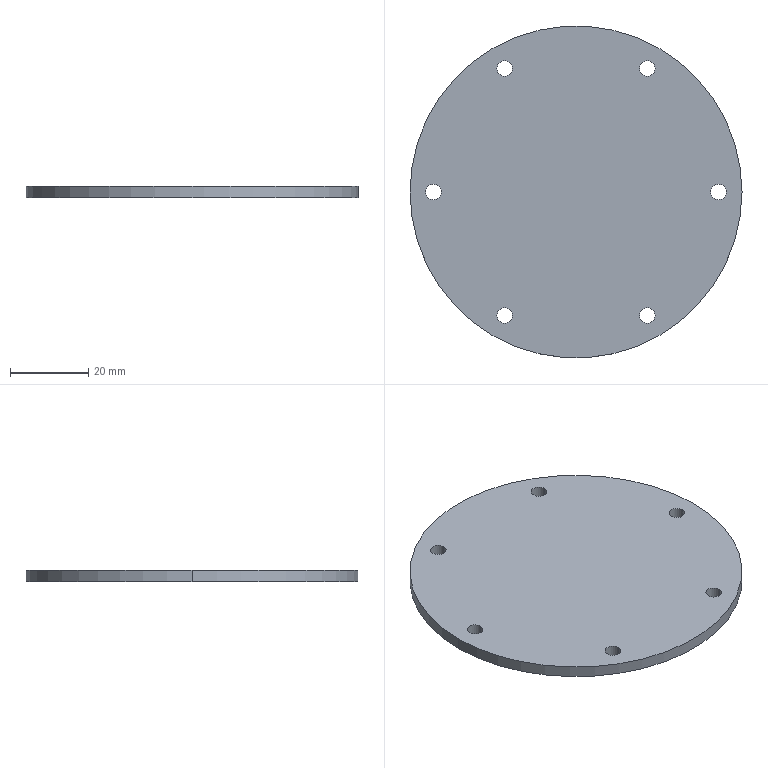Part | SolidWorks | features FlatPattern 1, SMBaseFlange 1, SheetMetal 1 | 1 solid | 16 faces | box 85 x 85 x 3 mm | volume 16797 mm3 | cylinder 14 | plane 2 | commonest cylinder face diameters 4 x12 85 x2
STEP:
#1=CARTESIAN_POINT('',(500.89,-193.14,3.));
#2=VERTEX_POINT('',#1);
#3=CARTESIAN_POINT('',(504.89,-193.14,3.));
#4=VERTEX_POINT('',#3);
#5=CARTESIAN_POINT('',(502.89,-193.14,3.));
#6=DIRECTION('',(0.,0.,1.));
#7=DIRECTION('',(1.,0.,0.));
#8=AXIS2_PLACEMENT_3D('',#5,#6,#7);
#9=CIRCLE('',#8,2.);
#10=EDGE_CURVE('',#2,#4,#9,.T.);
#11=ORIENTED_EDGE('',*,*,#10,.T.);
#12=CARTESIAN_POINT('',(504.89,-193.14,0.));
#13=VERTEX_POINT('',#12);
#14=CARTESIAN_POINT('',(504.89,-193.14,3.));
#15=DIRECTION('',(0.,0.,-1.));
#16=VECTOR('',#15,1000.);
#17=LINE('',#14,#16);
#18=EDGE_CURVE('',#4,#13,#17,.T.);
#19=ORIENTED_EDGE('',*,*,#18,.T.);
#20=CARTESIAN_POINT('',(500.89,-193.14,0.));
#21=VERTEX_POINT('',#20);
#22=CARTESIAN_POINT('',(502.89,-193.14,0.));
#23=DIRECTION('',(0.,0.,1.));
#24=DIRECTION('',(1.,0.,0.));
#25=AXIS2_PLACEMENT_3D('',#22,#23,#24);
#26=CIRCLE('',#25,2.);
#27=EDGE_CURVE('',#21,#13,#26,.T.);
#28=ORIENTED_EDGE('',*,*,#27,.F.);
#29=CARTESIAN_POINT('',(500.89,-193.14,3.));
#30=DIRECTION('',(0.,0.,-1.));
#31=VECTOR('',#30,1000.);
#32=LINE('',#29,#31);
#33=EDGE_CURVE('',#2,#21,#32,.T.);
#34=ORIENTED_EDGE('',*,*,#33,.F.);
#35=EDGE_LOOP('',(#11,#19,#28,#34));
#36=FACE_OUTER_BOUND('',#35,.T.);
#37=CARTESIAN_POINT('',(502.89,-193.14,3.));
#38=DIRECTION('',(0.,0.,-1.));
#39=DIRECTION('',(-1.,0.,0.));
#40=AXIS2_PLACEMENT_3D('',#37,#38,#39);
#41=CYLINDRICAL_SURFACE('',#40,2.);
#42=ADVANCED_FACE('',(#36),#41,.F.);
#43=CARTESIAN_POINT('',(464.39,-193.14,3.));
#44=VERTEX_POINT('',#43);
#45=CARTESIAN_POINT('',(468.39,-193.14,3.));
#46=VERTEX_POINT('',#45);
#47=CARTESIAN_POINT('',(466.39,-193.14,3.));
#48=DIRECTION('',(0.,0.,1.));
#49=DIRECTION('',(1.,0.,0.));
#50=AXIS2_PLACEMENT_3D('',#47,#48,#49);
#51=CIRCLE('',#50,2.);
#52=EDGE_CURVE('',#44,#46,#51,.T.);
#53=ORIENTED_EDGE('',*,*,#52,.T.);
#54=CARTESIAN_POINT('',(468.39,-193.14,0.));
#55=VERTEX_POINT('',#54);
#56=CARTESIAN_POINT('',(468.39,-193.14,3.));
#57=DIRECTION('',(0.,0.,-1.));
#58=VECTOR('',#57,1000.);
#59=LINE('',#56,#58);
#60=EDGE_CURVE('',#46,#55,#59,.T.);
#61=ORIENTED_EDGE('',*,*,#60,.T.);
#62=CARTESIAN_POINT('',(464.39,-193.14,0.));
#63=VERTEX_POINT('',#62);
#64=CARTESIAN_POINT('',(466.39,-193.14,0.));
#65=DIRECTION('',(0.,0.,1.));
#66=DIRECTION('',(1.,0.,0.));
#67=AXIS2_PLACEMENT_3D('',#64,#65,#66);
#68=CIRCLE('',#67,2.);
#69=EDGE_CURVE('',#63,#55,#68,.T.);
#70=ORIENTED_EDGE('',*,*,#69,.F.);
#71=CARTESIAN_POINT('',(464.39,-193.14,3.));
#72=DIRECTION('',(0.,0.,-1.));
#73=VECTOR('',#72,1000.);
#74=LINE('',#71,#73);
#75=EDGE_CURVE('',#44,#63,#74,.T.);
#76=ORIENTED_EDGE('',*,*,#75,.F.);
#77=EDGE_LOOP('',(#53,#61,#70,#76));
#78=FACE_OUTER_BOUND('',#77,.T.);
#79=CARTESIAN_POINT('',(466.39,-193.14,3.));
#80=DIRECTION('',(0.,0.,-1.));
#81=DIRECTION('',(-1.,0.,0.));
#82=AXIS2_PLACEMENT_3D('',#79,#80,#81);
#83=CYLINDRICAL_SURFACE('',#82,2.);
#84=ADVANCED_FACE('',(#78),#83,.F.);
#85=CARTESIAN_POINT('',(446.14,-224.75,3.));
#86=VERTEX_POINT('',#85);
#87=CARTESIAN_POINT('',(450.14,-224.75,3.));
#88=VERTEX_POINT('',#87);
#89=CARTESIAN_POINT('',(448.14,-224.75,3.));
#90=DIRECTION('',(0.,0.,1.));
#91=DIRECTION('',(1.,0.,0.));
#92=AXIS2_PLACEMENT_3D('',#89,#90,#91);
#93=CIRCLE('',#92,2.);
#94=EDGE_CURVE('',#86,#88,#93,.T.);
#95=ORIENTED_EDGE('',*,*,#94,.T.);
#96=CARTESIAN_POINT('',(450.14,-224.75,0.));
#97=VERTEX_POINT('',#96);
#98=CARTESIAN_POINT('',(450.14,-224.75,3.));
#99=DIRECTION('',(0.,0.,-1.));
#100=VECTOR('',#99,1000.);
#101=LINE('',#98,#100);
#102=EDGE_CURVE('',#88,#97,#101,.T.);
#103=ORIENTED_EDGE('',*,*,#102,.T.);
#104=CARTESIAN_POINT('',(446.14,-224.75,0.));
#105=VERTEX_POINT('',#104);
#106=CARTESIAN_POINT('',(448.14,-224.75,0.));
#107=DIRECTION('',(0.,0.,1.));
#108=DIRECTION('',(1.,0.,0.));
#109=AXIS2_PLACEMENT_3D('',#106,#107,#108);
#110=CIRCLE('',#109,2.);
#111=EDGE_CURVE('',#105,#97,#110,.T.);
#112=ORIENTED_EDGE('',*,*,#111,.F.);
#113=CARTESIAN_POINT('',(446.14,-224.75,3.));
#114=DIRECTION('',(0.,0.,-1.));
#115=VECTOR('',#114,1000.);
#116=LINE('',#113,#115);
#117=EDGE_CURVE('',#86,#105,#116,.T.);
#118=ORIENTED_EDGE('',*,*,#117,.F.);
#119=EDGE_LOOP('',(#95,#103,#112,#118));
#120=FACE_OUTER_BOUND('',#119,.T.);
#121=CARTESIAN_POINT('',(448.14,-224.75,3.));
#122=DIRECTION('',(0.,0.,-1.));
#123=DIRECTION('',(-1.,0.,0.));
#124=AXIS2_PLACEMENT_3D('',#121,#122,#123);
#125=CYLINDRICAL_SURFACE('',#124,2.);
#126=ADVANCED_FACE('',(#120),#125,.F.);
#127=CARTESIAN_POINT('',(464.39,-256.36,3.));
#128=VERTEX_POINT('',#127);
#129=CARTESIAN_POINT('',(468.39,-256.36,3.));
#130=VERTEX_POINT('',#129);
#131=CARTESIAN_POINT('',(466.39,-256.36,3.));
#132=DIRECTION('',(0.,0.,1.));
#133=DIRECTION('',(1.,0.,0.));
#134=AXIS2_PLACEMENT_3D('',#131,#132,#133);
#135=CIRCLE('',#134,2.);
#136=EDGE_CURVE('',#128,#130,#135,.T.);
#137=ORIENTED_EDGE('',*,*,#136,.T.);
#138=CARTESIAN_POINT('',(468.39,-256.36,0.));
#139=VERTEX_POINT('',#138);
#140=CARTESIAN_POINT('',(468.39,-256.36,3.));
#141=DIRECTION('',(0.,0.,-1.));
#142=VECTOR('',#141,1000.);
#143=LINE('',#140,#142);
#144=EDGE_CURVE('',#130,#139,#143,.T.);
#145=ORIENTED_EDGE('',*,*,#144,.T.);
#146=CARTESIAN_POINT('',(464.39,-256.36,0.));
#147=VERTEX_POINT('',#146);
#148=CARTESIAN_POINT('',(466.39,-256.36,0.));
#149=DIRECTION('',(0.,0.,1.));
#150=DIRECTION('',(1.,0.,0.));
#151=AXIS2_PLACEMENT_3D('',#148,#149,#150);
#152=CIRCLE('',#151,2.);
#153=EDGE_CURVE('',#147,#139,#152,.T.);
#154=ORIENTED_EDGE('',*,*,#153,.F.);
#155=CARTESIAN_POINT('',(464.39,-256.36,3.));
#156=DIRECTION('',(0.,0.,-1.));
#157=VECTOR('',#156,1000.);
#158=LINE('',#155,#157);
#159=EDGE_CURVE('',#128,#147,#158,.T.);
#160=ORIENTED_EDGE('',*,*,#159,.F.);
#161=EDGE_LOOP('',(#137,#145,#154,#160));
#162=FACE_OUTER_BOUND('',#161,.T.);
#163=CARTESIAN_POINT('',(466.39,-256.36,3.));
#164=DIRECTION('',(0.,0.,-1.));
#165=DIRECTION('',(-1.,0.,0.));
#166=AXIS2_PLACEMENT_3D('',#163,#164,#165);
#167=CYLINDRICAL_SURFACE('',#166,2.);
#168=ADVANCED_FACE('',(#162),#167,.F.);
#169=CARTESIAN_POINT('',(500.89,-256.36,3.));
#170=VERTEX_POINT('',#169);
#171=CARTESIAN_POINT('',(504.89,-256.36,3.));
#172=VERTEX_POINT('',#171);
#173=CARTESIAN_POINT('',(502.89,-256.36,3.));
#174=DIRECTION('',(0.,0.,1.));
#175=DIRECTION('',(1.,0.,0.));
#176=AXIS2_PLACEMENT_3D('',#173,#174,#175);
#177=CIRCLE('',#176,2.);
#178=EDGE_CURVE('',#170,#172,#177,.T.);
#179=ORIENTED_EDGE('',*,*,#178,.T.);
#180=CARTESIAN_POINT('',(504.89,-256.36,0.));
#181=VERTEX_POINT('',#180);
#182=CARTESIAN_POINT('',(504.89,-256.36,3.));
#183=DIRECTION('',(0.,0.,-1.));
#184=VECTOR('',#183,1000.);
#185=LINE('',#182,#184);
#186=EDGE_CURVE('',#172,#181,#185,.T.);
#187=ORIENTED_EDGE('',*,*,#186,.T.);
#188=CARTESIAN_POINT('',(500.89,-256.36,0.));
#189=VERTEX_POINT('',#188);
#190=CARTESIAN_POINT('',(502.89,-256.36,0.));
#191=DIRECTION('',(0.,0.,1.));
#192=DIRECTION('',(1.,0.,0.));
#193=AXIS2_PLACEMENT_3D('',#190,#191,#192);
#194=CIRCLE('',#193,2.);
#195=EDGE_CURVE('',#189,#181,#194,.T.);
#196=ORIENTED_EDGE('',*,*,#195,.F.);
#197=CARTESIAN_POINT('',(500.89,-256.36,3.));
#198=DIRECTION('',(0.,0.,-1.));
#199=VECTOR('',#198,1000.);
#200=LINE('',#197,#199);
#201=EDGE_CURVE('',#170,#189,#200,.T.);
#202=ORIENTED_EDGE('',*,*,#201,.F.);
#203=EDGE_LOOP('',(#179,#187,#196,#202));
#204=FACE_OUTER_BOUND('',#203,.T.);
#205=CARTESIAN_POINT('',(502.89,-256.36,3.));
#206=DIRECTION('',(0.,0.,-1.));
#207=DIRECTION('',(-1.,0.,0.));
#208=AXIS2_PLACEMENT_3D('',#205,#206,#207);
#209=CYLINDRICAL_SURFACE('',#208,2.);
#210=ADVANCED_FACE('',(#204),#209,.F.);
#211=CARTESIAN_POINT('',(519.14,-224.75,3.));
#212=VERTEX_POINT('',#211);
#213=CARTESIAN_POINT('',(523.14,-224.75,3.));
#214=VERTEX_POINT('',#213);
#215=CARTESIAN_POINT('',(521.14,-224.75,3.));
#216=DIRECTION('',(0.,0.,1.));
#217=DIRECTION('',(1.,0.,0.));
#218=AXIS2_PLACEMENT_3D('',#215,#216,#217);
#219=CIRCLE('',#218,2.);
#220=EDGE_CURVE('',#212,#214,#219,.T.);
#221=ORIENTED_EDGE('',*,*,#220,.T.);
#222=CARTESIAN_POINT('',(523.14,-224.75,0.));
#223=VERTEX_POINT('',#222);
#224=CARTESIAN_POINT('',(523.14,-224.75,3.));
#225=DIRECTION('',(0.,0.,-1.));
#226=VECTOR('',#225,1000.);
#227=LINE('',#224,#226);
#228=EDGE_CURVE('',#214,#223,#227,.T.);
#229=ORIENTED_EDGE('',*,*,#228,.T.);
#230=CARTESIAN_POINT('',(519.14,-224.75,0.));
#231=VERTEX_POINT('',#230);
#232=CARTESIAN_POINT('',(521.14,-224.75,0.));
#233=DIRECTION('',(0.,0.,1.));
#234=DIRECTION('',(1.,0.,0.));
#235=AXIS2_PLACEMENT_3D('',#232,#233,#234);
#236=CIRCLE('',#235,2.);
#237=EDGE_CURVE('',#231,#223,#236,.T.);
#238=ORIENTED_EDGE('',*,*,#237,.F.);
#239=CARTESIAN_POINT('',(519.14,-224.75,3.));
#240=DIRECTION('',(0.,0.,-1.));
#241=VECTOR('',#240,1000.);
#242=LINE('',#239,#241);
#243=EDGE_CURVE('',#212,#231,#242,.T.);
#244=ORIENTED_EDGE('',*,*,#243,.F.);
#245=EDGE_LOOP('',(#221,#229,#238,#244));
#246=FACE_OUTER_BOUND('',#245,.T.);
#247=CARTESIAN_POINT('',(521.14,-224.75,3.));
#248=DIRECTION('',(0.,0.,-1.));
#249=DIRECTION('',(-1.,0.,0.));
#250=AXIS2_PLACEMENT_3D('',#247,#248,#249);
#251=CYLINDRICAL_SURFACE('',#250,2.);
#252=ADVANCED_FACE('',(#246),#251,.F.);
#253=CARTESIAN_POINT('',(527.14,-224.75,3.));
#254=VERTEX_POINT('',#253);
#255=CARTESIAN_POINT('',(442.14,-224.75,3.));
#256=VERTEX_POINT('',#255);
#257=CARTESIAN_POINT('',(484.64,-224.75,3.));
#258=DIRECTION('',(0.,0.,1.));
#259=DIRECTION('',(1.,0.,0.));
#260=AXIS2_PLACEMENT_3D('',#257,#258,#259);
#261=CIRCLE('',#260,42.5);
#262=EDGE_CURVE('',#254,#256,#261,.T.);
#263=ORIENTED_EDGE('',*,*,#262,.F.);
#264=CARTESIAN_POINT('',(527.14,-224.75,0.));
#265=VERTEX_POINT('',#264);
#266=CARTESIAN_POINT('',(527.14,-224.75,3.));
#267=DIRECTION('',(0.,0.,-1.));
#268=VECTOR('',#267,1000.);
#269=LINE('',#266,#268);
#270=EDGE_CURVE('',#254,#265,#269,.T.);
#271=ORIENTED_EDGE('',*,*,#270,.T.);
#272=CARTESIAN_POINT('',(442.14,-224.75,0.));
#273=VERTEX_POINT('',#272);
#274=CARTESIAN_POINT('',(484.64,-224.75,0.));
#275=DIRECTION('',(0.,0.,1.));
#276=DIRECTION('',(1.,0.,0.));
#277=AXIS2_PLACEMENT_3D('',#274,#275,#276);
#278=CIRCLE('',#277,42.5);
#279=EDGE_CURVE('',#265,#273,#278,.T.);
#280=ORIENTED_EDGE('',*,*,#279,.T.);
#281=CARTESIAN_POINT('',(442.14,-224.75,3.));
#282=DIRECTION('',(0.,0.,-1.));
#283=VECTOR('',#282,1000.);
#284=LINE('',#281,#283);
#285=EDGE_CURVE('',#256,#273,#284,.T.);
#286=ORIENTED_EDGE('',*,*,#285,.F.);
#287=EDGE_LOOP('',(#263,#271,#280,#286));
#288=FACE_OUTER_BOUND('',#287,.T.);
#289=CARTESIAN_POINT('',(484.64,-224.75,3.));
#290=DIRECTION('',(0.,0.,-1.));
#291=DIRECTION('',(-1.,0.,0.));
#292=AXIS2_PLACEMENT_3D('',#289,#290,#291);
#293=CYLINDRICAL_SURFACE('',#292,42.5);
#294=ADVANCED_FACE('',(#288),#293,.T.);
#295=ORIENTED_EDGE('',*,*,#52,.F.);
#296=CARTESIAN_POINT('',(466.39,-193.14,3.));
#297=DIRECTION('',(0.,0.,1.));
#298=DIRECTION('',(1.,0.,0.));
#299=AXIS2_PLACEMENT_3D('',#296,#297,#298);
#300=CIRCLE('',#299,2.);
#301=EDGE_CURVE('',#46,#44,#300,.T.);
#302=ORIENTED_EDGE('',*,*,#301,.F.);
#303=EDGE_LOOP('',(#295,#302));
#304=FACE_BOUND('',#303,.T.);
#305=ORIENTED_EDGE('',*,*,#136,.F.);
#306=CARTESIAN_POINT('',(466.39,-256.36,3.));
#307=DIRECTION('',(0.,0.,1.));
#308=DIRECTION('',(1.,0.,0.));
#309=AXIS2_PLACEMENT_3D('',#306,#307,#308);
#310=CIRCLE('',#309,2.);
#311=EDGE_CURVE('',#130,#128,#310,.T.);
#312=ORIENTED_EDGE('',*,*,#311,.F.);
#313=EDGE_LOOP('',(#305,#312));
#314=FACE_BOUND('',#313,.T.);
#315=ORIENTED_EDGE('',*,*,#220,.F.);
#316=CARTESIAN_POINT('',(521.14,-224.75,3.));
#317=DIRECTION('',(0.,0.,1.));
#318=DIRECTION('',(1.,0.,0.));
#319=AXIS2_PLACEMENT_3D('',#316,#317,#318);
#320=CIRCLE('',#319,2.);
#321=EDGE_CURVE('',#214,#212,#320,.T.);
#322=ORIENTED_EDGE('',*,*,#321,.F.);
#323=EDGE_LOOP('',(#315,#322));
#324=FACE_BOUND('',#323,.T.);
#325=CARTESIAN_POINT('',(484.64,-224.75,3.));
#326=DIRECTION('',(0.,0.,1.));
#327=DIRECTION('',(1.,0.,0.));
#328=AXIS2_PLACEMENT_3D('',#325,#326,#327);
#329=CIRCLE('',#328,42.5);
#330=EDGE_CURVE('',#256,#254,#329,.T.);
#331=ORIENTED_EDGE('',*,*,#330,.T.);
#332=ORIENTED_EDGE('',*,*,#262,.T.);
#333=EDGE_LOOP('',(#331,#332));
#334=FACE_OUTER_BOUND('',#333,.T.);
#335=ORIENTED_EDGE('',*,*,#178,.F.);
#336=CARTESIAN_POINT('',(502.89,-256.36,3.));
#337=DIRECTION('',(0.,0.,1.));
#338=DIRECTION('',(1.,0.,0.));
#339=AXIS2_PLACEMENT_3D('',#336,#337,#338);
#340=CIRCLE('',#339,2.);
#341=EDGE_CURVE('',#172,#170,#340,.T.);
#342=ORIENTED_EDGE('',*,*,#341,.F.);
#343=EDGE_LOOP('',(#335,#342));
#344=FACE_BOUND('',#343,.T.);
#345=ORIENTED_EDGE('',*,*,#94,.F.);
#346=CARTESIAN_POINT('',(448.14,-224.75,3.));
#347=DIRECTION('',(0.,0.,1.));
#348=DIRECTION('',(1.,0.,0.));
#349=AXIS2_PLACEMENT_3D('',#346,#347,#348);
#350=CIRCLE('',#349,2.);
#351=EDGE_CURVE('',#88,#86,#350,.T.);
#352=ORIENTED_EDGE('',*,*,#351,.F.);
#353=EDGE_LOOP('',(#345,#352));
#354=FACE_BOUND('',#353,.T.);
#355=ORIENTED_EDGE('',*,*,#10,.F.);
#356=CARTESIAN_POINT('',(502.89,-193.14,3.));
#357=DIRECTION('',(0.,0.,1.));
#358=DIRECTION('',(1.,0.,0.));
#359=AXIS2_PLACEMENT_3D('',#356,#357,#358);
#360=CIRCLE('',#359,2.);
#361=EDGE_CURVE('',#4,#2,#360,.T.);
#362=ORIENTED_EDGE('',*,*,#361,.F.);
#363=EDGE_LOOP('',(#355,#362));
#364=FACE_BOUND('',#363,.T.);
#365=CARTESIAN_POINT('',(484.64,-224.75,3.));
#366=DIRECTION('',(0.,0.,1.));
#367=DIRECTION('',(1.,0.,0.));
#368=AXIS2_PLACEMENT_3D('',#365,#366,#367);
#369=PLANE('',#368);
#370=ADVANCED_FACE('',(#304,#314,#324,#334,#344,#354,#364),#369,.T.);
#371=CARTESIAN_POINT('',(484.64,-224.75,0.));
#372=DIRECTION('',(0.,0.,1.));
#373=DIRECTION('',(1.,0.,0.));
#374=AXIS2_PLACEMENT_3D('',#371,#372,#373);
#375=CIRCLE('',#374,42.5);
#376=EDGE_CURVE('',#273,#265,#375,.T.);
#377=ORIENTED_EDGE('',*,*,#376,.F.);
#378=ORIENTED_EDGE('',*,*,#279,.F.);
#379=EDGE_LOOP('',(#377,#378));
#380=FACE_OUTER_BOUND('',#379,.T.);
#381=ORIENTED_EDGE('',*,*,#237,.T.);
#382=CARTESIAN_POINT('',(521.14,-224.75,0.));
#383=DIRECTION('',(0.,0.,1.));
#384=DIRECTION('',(1.,0.,0.));
#385=AXIS2_PLACEMENT_3D('',#382,#383,#384);
#386=CIRCLE('',#385,2.);
#387=EDGE_CURVE('',#223,#231,#386,.T.);
#388=ORIENTED_EDGE('',*,*,#387,.T.);
#389=EDGE_LOOP('',(#381,#388));
#390=FACE_BOUND('',#389,.T.);
#391=ORIENTED_EDGE('',*,*,#195,.T.);
#392=CARTESIAN_POINT('',(502.89,-256.36,0.));
#393=DIRECTION('',(0.,0.,1.));
#394=DIRECTION('',(1.,0.,0.));
#395=AXIS2_PLACEMENT_3D('',#392,#393,#394);
#396=CIRCLE('',#395,2.);
#397=EDGE_CURVE('',#181,#189,#396,.T.);
#398=ORIENTED_EDGE('',*,*,#397,.T.);
#399=EDGE_LOOP('',(#391,#398));
#400=FACE_BOUND('',#399,.T.);
#401=ORIENTED_EDGE('',*,*,#153,.T.);
#402=CARTESIAN_POINT('',(466.39,-256.36,0.));
#403=DIRECTION('',(0.,0.,1.));
#404=DIRECTION('',(1.,0.,0.));
#405=AXIS2_PLACEMENT_3D('',#402,#403,#404);
#406=CIRCLE('',#405,2.);
#407=EDGE_CURVE('',#139,#147,#406,.T.);
#408=ORIENTED_EDGE('',*,*,#407,.T.);
#409=EDGE_LOOP('',(#401,#408));
#410=FACE_BOUND('',#409,.T.);
#411=ORIENTED_EDGE('',*,*,#111,.T.);
#412=CARTESIAN_POINT('',(448.14,-224.75,0.));
#413=DIRECTION('',(0.,0.,1.));
#414=DIRECTION('',(1.,0.,0.));
#415=AXIS2_PLACEMENT_3D('',#412,#413,#414);
#416=CIRCLE('',#415,2.);
#417=EDGE_CURVE('',#97,#105,#416,.T.);
#418=ORIENTED_EDGE('',*,*,#417,.T.);
#419=EDGE_LOOP('',(#411,#418));
#420=FACE_BOUND('',#419,.T.);
#421=ORIENTED_EDGE('',*,*,#69,.T.);
#422=CARTESIAN_POINT('',(466.39,-193.14,0.));
#423=DIRECTION('',(0.,0.,1.));
#424=DIRECTION('',(1.,0.,0.));
#425=AXIS2_PLACEMENT_3D('',#422,#423,#424);
#426=CIRCLE('',#425,2.);
#427=EDGE_CURVE('',#55,#63,#426,.T.);
#428=ORIENTED_EDGE('',*,*,#427,.T.);
#429=EDGE_LOOP('',(#421,#428));
#430=FACE_BOUND('',#429,.T.);
#431=ORIENTED_EDGE('',*,*,#27,.T.);
#432=CARTESIAN_POINT('',(502.89,-193.14,0.));
#433=DIRECTION('',(0.,0.,1.));
#434=DIRECTION('',(1.,0.,0.));
#435=AXIS2_PLACEMENT_3D('',#432,#433,#434);
#436=CIRCLE('',#435,2.);
#437=EDGE_CURVE('',#13,#21,#436,.T.);
#438=ORIENTED_EDGE('',*,*,#437,.T.);
#439=EDGE_LOOP('',(#431,#438));
#440=FACE_BOUND('',#439,.T.);
#441=CARTESIAN_POINT('',(484.64,-224.75,0.));
#442=DIRECTION('',(0.,0.,1.));
#443=DIRECTION('',(1.,0.,0.));
#444=AXIS2_PLACEMENT_3D('',#441,#442,#443);
#445=PLANE('',#444);
#446=ADVANCED_FACE('',(#380,#390,#400,#410,#420,#430,#440),#445,.F.);
#447=ORIENTED_EDGE('',*,*,#270,.F.);
#448=ORIENTED_EDGE('',*,*,#330,.F.);
#449=ORIENTED_EDGE('',*,*,#285,.T.);
#450=ORIENTED_EDGE('',*,*,#376,.T.);
#451=EDGE_LOOP('',(#447,#448,#449,#450));
#452=FACE_OUTER_BOUND('',#451,.T.);
#453=CARTESIAN_POINT('',(484.64,-224.75,3.));
#454=DIRECTION('',(0.,0.,-1.));
#455=DIRECTION('',(-1.,0.,0.));
#456=AXIS2_PLACEMENT_3D('',#453,#454,#455);
#457=CYLINDRICAL_SURFACE('',#456,42.5);
#458=ADVANCED_FACE('',(#452),#457,.T.);
#459=ORIENTED_EDGE('',*,*,#228,.F.);
#460=ORIENTED_EDGE('',*,*,#321,.T.);
#461=ORIENTED_EDGE('',*,*,#243,.T.);
#462=ORIENTED_EDGE('',*,*,#387,.F.);
#463=EDGE_LOOP('',(#459,#460,#461,#462));
#464=FACE_OUTER_BOUND('',#463,.T.);
#465=CARTESIAN_POINT('',(521.14,-224.75,3.));
#466=DIRECTION('',(0.,0.,-1.));
#467=DIRECTION('',(-1.,0.,0.));
#468=AXIS2_PLACEMENT_3D('',#465,#466,#467);
#469=CYLINDRICAL_SURFACE('',#468,2.);
#470=ADVANCED_FACE('',(#464),#469,.F.);
#471=ORIENTED_EDGE('',*,*,#186,.F.);
#472=ORIENTED_EDGE('',*,*,#341,.T.);
#473=ORIENTED_EDGE('',*,*,#201,.T.);
#474=ORIENTED_EDGE('',*,*,#397,.F.);
#475=EDGE_LOOP('',(#471,#472,#473,#474));
#476=FACE_OUTER_BOUND('',#475,.T.);
#477=CARTESIAN_POINT('',(502.89,-256.36,3.));
#478=DIRECTION('',(0.,0.,-1.));
#479=DIRECTION('',(-1.,0.,0.));
#480=AXIS2_PLACEMENT_3D('',#477,#478,#479);
#481=CYLINDRICAL_SURFACE('',#480,2.);
#482=ADVANCED_FACE('',(#476),#481,.F.);
#483=ORIENTED_EDGE('',*,*,#144,.F.);
#484=ORIENTED_EDGE('',*,*,#311,.T.);
#485=ORIENTED_EDGE('',*,*,#159,.T.);
#486=ORIENTED_EDGE('',*,*,#407,.F.);
#487=EDGE_LOOP('',(#483,#484,#485,#486));
#488=FACE_OUTER_BOUND('',#487,.T.);
#489=CARTESIAN_POINT('',(466.39,-256.36,3.));
#490=DIRECTION('',(0.,0.,-1.));
#491=DIRECTION('',(-1.,0.,0.));
#492=AXIS2_PLACEMENT_3D('',#489,#490,#491);
#493=CYLINDRICAL_SURFACE('',#492,2.);
#494=ADVANCED_FACE('',(#488),#493,.F.);
#495=ORIENTED_EDGE('',*,*,#102,.F.);
#496=ORIENTED_EDGE('',*,*,#351,.T.);
#497=ORIENTED_EDGE('',*,*,#117,.T.);
#498=ORIENTED_EDGE('',*,*,#417,.F.);
#499=EDGE_LOOP('',(#495,#496,#497,#498));
#500=FACE_OUTER_BOUND('',#499,.T.);
#501=CARTESIAN_POINT('',(448.14,-224.75,3.));
#502=DIRECTION('',(0.,0.,-1.));
#503=DIRECTION('',(-1.,0.,0.));
#504=AXIS2_PLACEMENT_3D('',#501,#502,#503);
#505=CYLINDRICAL_SURFACE('',#504,2.);
#506=ADVANCED_FACE('',(#500),#505,.F.);
#507=ORIENTED_EDGE('',*,*,#60,.F.);
#508=ORIENTED_EDGE('',*,*,#301,.T.);
#509=ORIENTED_EDGE('',*,*,#75,.T.);
#510=ORIENTED_EDGE('',*,*,#427,.F.);
#511=EDGE_LOOP('',(#507,#508,#509,#510));
#512=FACE_OUTER_BOUND('',#511,.T.);
#513=CARTESIAN_POINT('',(466.39,-193.14,3.));
#514=DIRECTION('',(0.,0.,-1.));
#515=DIRECTION('',(-1.,0.,0.));
#516=AXIS2_PLACEMENT_3D('',#513,#514,#515);
#517=CYLINDRICAL_SURFACE('',#516,2.);
#518=ADVANCED_FACE('',(#512),#517,.F.);
#519=ORIENTED_EDGE('',*,*,#18,.F.);
#520=ORIENTED_EDGE('',*,*,#361,.T.);
#521=ORIENTED_EDGE('',*,*,#33,.T.);
#522=ORIENTED_EDGE('',*,*,#437,.F.);
#523=EDGE_LOOP('',(#519,#520,#521,#522));
#524=FACE_OUTER_BOUND('',#523,.T.);
#525=CARTESIAN_POINT('',(502.89,-193.14,3.));
#526=DIRECTION('',(0.,0.,-1.));
#527=DIRECTION('',(-1.,0.,0.));
#528=AXIS2_PLACEMENT_3D('',#525,#526,#527);
#529=CYLINDRICAL_SURFACE('',#528,2.);
#530=ADVANCED_FACE('',(#524),#529,.F.);
#531=CLOSED_SHELL('',(#42,#84,#126,#168,#210,#252,#294,#370,#446,#458,#470,#482,#494,#506,#518,#530));
#532=MANIFOLD_SOLID_BREP('',#531);
#533=CARTESIAN_POINT('',(0.,0.,0.));
#534=DIRECTION('',(0.,0.,1.));
#535=DIRECTION('',(1.,0.,0.));
#536=AXIS2_PLACEMENT_3D('',#533,#534,#535);
#537=(LENGTH_UNIT()NAMED_UNIT(*)SI_UNIT(.MILLI.,.METRE.));
#538=UNCERTAINTY_MEASURE_WITH_UNIT(LENGTH_MEASURE(0.00001),#537,'','');
#539=(NAMED_UNIT(*)PLANE_ANGLE_UNIT()SI_UNIT($,.RADIAN.));
#540=(NAMED_UNIT(*)SI_UNIT($,.STERADIAN.)SOLID_ANGLE_UNIT());
#541=(GEOMETRIC_REPRESENTATION_CONTEXT(3)GLOBAL_UNCERTAINTY_ASSIGNED_CONTEXT((#538))GLOBAL_UNIT_ASSIGNED_CONTEXT((#537,#539,#540))REPRESENTATION_CONTEXT('',''));
#542=ADVANCED_BREP_SHAPE_REPRESENTATION('',(#532,#536),#541);